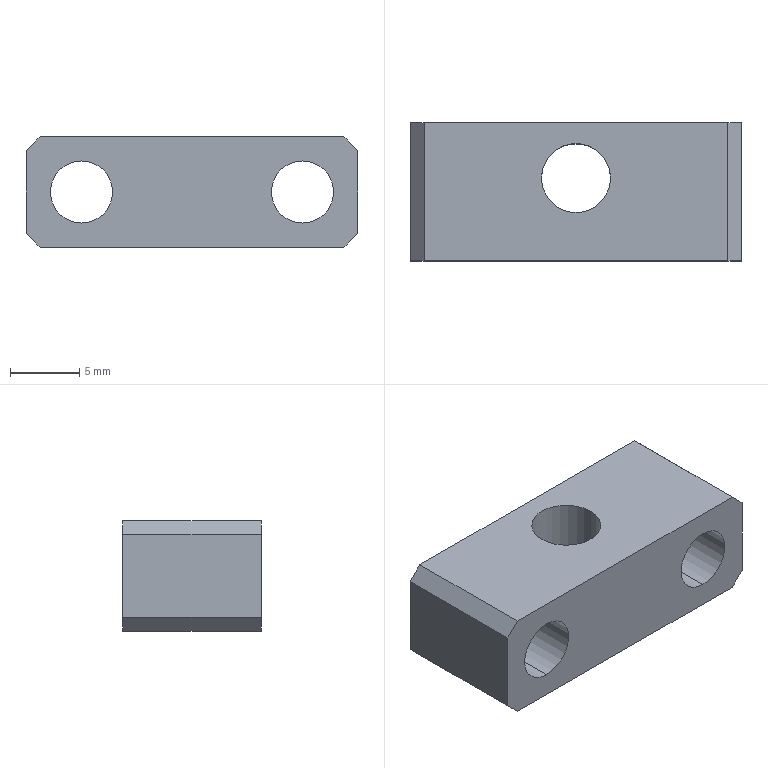Part | SolidWorks | features HoleWzd 2, Chamfer 1, Extrusion 1 | 1 solid | 16 faces | box 24 x 10 x 8 mm | volume 1425 mm3 | plane 10 | cylinder 6 | commonest cylinder face diameters 4.5 x4 5 x2
STEP:
#1=CARTESIAN_POINT('',(-2.5,1.,-4.));
#2=VERTEX_POINT('',#1);
#3=CARTESIAN_POINT('',(2.5,1.,-4.));
#4=VERTEX_POINT('',#3);
#5=CARTESIAN_POINT('',(0.,1.,-4.));
#6=DIRECTION('',(0.,0.,1.));
#7=DIRECTION('',(1.,0.,0.));
#8=AXIS2_PLACEMENT_3D('',#5,#6,#7);
#9=CIRCLE('',#8,2.5);
#10=EDGE_CURVE('',#2,#4,#9,.T.);
#11=ORIENTED_EDGE('',*,*,#10,.F.);
#12=CARTESIAN_POINT('',(-2.5,1.,4.));
#13=VERTEX_POINT('',#12);
#14=CARTESIAN_POINT('',(-2.5,1.,4.));
#15=DIRECTION('',(0.,0.,1.));
#16=VECTOR('',#15,1000.);
#17=LINE('',#14,#16);
#18=EDGE_CURVE('',#2,#13,#17,.T.);
#19=ORIENTED_EDGE('',*,*,#18,.T.);
#20=CARTESIAN_POINT('',(2.5,1.,4.));
#21=VERTEX_POINT('',#20);
#22=CARTESIAN_POINT('',(0.,1.,4.));
#23=DIRECTION('',(0.,0.,1.));
#24=DIRECTION('',(1.,0.,0.));
#25=AXIS2_PLACEMENT_3D('',#22,#23,#24);
#26=CIRCLE('',#25,2.5);
#27=EDGE_CURVE('',#13,#21,#26,.T.);
#28=ORIENTED_EDGE('',*,*,#27,.T.);
#29=CARTESIAN_POINT('',(2.5,1.,4.));
#30=DIRECTION('',(0.,0.,1.));
#31=VECTOR('',#30,1000.);
#32=LINE('',#29,#31);
#33=EDGE_CURVE('',#4,#21,#32,.T.);
#34=ORIENTED_EDGE('',*,*,#33,.F.);
#35=EDGE_LOOP('',(#11,#19,#28,#34));
#36=FACE_OUTER_BOUND('',#35,.T.);
#37=CARTESIAN_POINT('',(0.,1.,4.));
#38=DIRECTION('',(0.,0.,1.));
#39=DIRECTION('',(1.,0.,0.));
#40=AXIS2_PLACEMENT_3D('',#37,#38,#39);
#41=CYLINDRICAL_SURFACE('',#40,2.5);
#42=ADVANCED_FACE('',(#36),#41,.F.);
#43=CARTESIAN_POINT('',(-8.,-5.,-2.25));
#44=VERTEX_POINT('',#43);
#45=CARTESIAN_POINT('',(-8.,-5.,2.25));
#46=VERTEX_POINT('',#45);
#47=CARTESIAN_POINT('',(-8.,-5.,0.));
#48=DIRECTION('',(0.,1.,0.));
#49=DIRECTION('',(0.,0.,1.));
#50=AXIS2_PLACEMENT_3D('',#47,#48,#49);
#51=CIRCLE('',#50,2.25);
#52=EDGE_CURVE('',#44,#46,#51,.T.);
#53=ORIENTED_EDGE('',*,*,#52,.F.);
#54=CARTESIAN_POINT('',(-8.,5.,-2.25));
#55=VERTEX_POINT('',#54);
#56=CARTESIAN_POINT('',(-8.,5.,-2.25));
#57=DIRECTION('',(0.,1.,0.));
#58=VECTOR('',#57,1000.);
#59=LINE('',#56,#58);
#60=EDGE_CURVE('',#44,#55,#59,.T.);
#61=ORIENTED_EDGE('',*,*,#60,.T.);
#62=CARTESIAN_POINT('',(-8.,5.,2.25));
#63=VERTEX_POINT('',#62);
#64=CARTESIAN_POINT('',(-8.,5.,0.));
#65=DIRECTION('',(0.,1.,0.));
#66=DIRECTION('',(0.,0.,1.));
#67=AXIS2_PLACEMENT_3D('',#64,#65,#66);
#68=CIRCLE('',#67,2.25);
#69=EDGE_CURVE('',#55,#63,#68,.T.);
#70=ORIENTED_EDGE('',*,*,#69,.T.);
#71=CARTESIAN_POINT('',(-8.,5.,2.25));
#72=DIRECTION('',(0.,1.,0.));
#73=VECTOR('',#72,1000.);
#74=LINE('',#71,#73);
#75=EDGE_CURVE('',#46,#63,#74,.T.);
#76=ORIENTED_EDGE('',*,*,#75,.F.);
#77=EDGE_LOOP('',(#53,#61,#70,#76));
#78=FACE_OUTER_BOUND('',#77,.T.);
#79=CARTESIAN_POINT('',(-8.,5.,0.));
#80=DIRECTION('',(0.,1.,0.));
#81=DIRECTION('',(0.,0.,1.));
#82=AXIS2_PLACEMENT_3D('',#79,#80,#81);
#83=CYLINDRICAL_SURFACE('',#82,2.25);
#84=ADVANCED_FACE('',(#78),#83,.F.);
#85=CARTESIAN_POINT('',(8.,-5.,-2.25));
#86=VERTEX_POINT('',#85);
#87=CARTESIAN_POINT('',(8.,-5.,2.25));
#88=VERTEX_POINT('',#87);
#89=CARTESIAN_POINT('',(8.,-5.,0.));
#90=DIRECTION('',(0.,1.,0.));
#91=DIRECTION('',(0.,0.,1.));
#92=AXIS2_PLACEMENT_3D('',#89,#90,#91);
#93=CIRCLE('',#92,2.25);
#94=EDGE_CURVE('',#86,#88,#93,.T.);
#95=ORIENTED_EDGE('',*,*,#94,.F.);
#96=CARTESIAN_POINT('',(8.,5.,-2.25));
#97=VERTEX_POINT('',#96);
#98=CARTESIAN_POINT('',(8.,5.,-2.25));
#99=DIRECTION('',(0.,1.,0.));
#100=VECTOR('',#99,1000.);
#101=LINE('',#98,#100);
#102=EDGE_CURVE('',#86,#97,#101,.T.);
#103=ORIENTED_EDGE('',*,*,#102,.T.);
#104=CARTESIAN_POINT('',(8.,5.,2.25));
#105=VERTEX_POINT('',#104);
#106=CARTESIAN_POINT('',(8.,5.,0.));
#107=DIRECTION('',(0.,1.,0.));
#108=DIRECTION('',(0.,0.,1.));
#109=AXIS2_PLACEMENT_3D('',#106,#107,#108);
#110=CIRCLE('',#109,2.25);
#111=EDGE_CURVE('',#97,#105,#110,.T.);
#112=ORIENTED_EDGE('',*,*,#111,.T.);
#113=CARTESIAN_POINT('',(8.,5.,2.25));
#114=DIRECTION('',(0.,1.,0.));
#115=VECTOR('',#114,1000.);
#116=LINE('',#113,#115);
#117=EDGE_CURVE('',#88,#105,#116,.T.);
#118=ORIENTED_EDGE('',*,*,#117,.F.);
#119=EDGE_LOOP('',(#95,#103,#112,#118));
#120=FACE_OUTER_BOUND('',#119,.T.);
#121=CARTESIAN_POINT('',(8.,5.,0.));
#122=DIRECTION('',(0.,1.,0.));
#123=DIRECTION('',(0.,0.,1.));
#124=AXIS2_PLACEMENT_3D('',#121,#122,#123);
#125=CYLINDRICAL_SURFACE('',#124,2.25);
#126=ADVANCED_FACE('',(#120),#125,.F.);
#127=CARTESIAN_POINT('',(12.,-5.,3.));
#128=VERTEX_POINT('',#127);
#129=CARTESIAN_POINT('',(12.,-5.,-3.));
#130=VERTEX_POINT('',#129);
#131=CARTESIAN_POINT('',(12.,-5.,4.));
#132=DIRECTION('',(0.,0.,-1.));
#133=VECTOR('',#132,1000.);
#134=LINE('',#131,#133);
#135=EDGE_CURVE('',#128,#130,#134,.T.);
#136=ORIENTED_EDGE('',*,*,#135,.T.);
#137=CARTESIAN_POINT('',(12.,5.,-3.));
#138=VERTEX_POINT('',#137);
#139=CARTESIAN_POINT('',(12.,5.,-3.));
#140=DIRECTION('',(0.,1.,0.));
#141=VECTOR('',#140,1000.);
#142=LINE('',#139,#141);
#143=EDGE_CURVE('',#130,#138,#142,.T.);
#144=ORIENTED_EDGE('',*,*,#143,.T.);
#145=CARTESIAN_POINT('',(12.,5.,3.));
#146=VERTEX_POINT('',#145);
#147=CARTESIAN_POINT('',(12.,5.,4.));
#148=DIRECTION('',(0.,0.,-1.));
#149=VECTOR('',#148,1000.);
#150=LINE('',#147,#149);
#151=EDGE_CURVE('',#146,#138,#150,.T.);
#152=ORIENTED_EDGE('',*,*,#151,.F.);
#153=CARTESIAN_POINT('',(12.,-5.,3.));
#154=DIRECTION('',(0.,-1.,0.));
#155=VECTOR('',#154,1000.);
#156=LINE('',#153,#155);
#157=EDGE_CURVE('',#146,#128,#156,.T.);
#158=ORIENTED_EDGE('',*,*,#157,.T.);
#159=EDGE_LOOP('',(#136,#144,#152,#158));
#160=FACE_OUTER_BOUND('',#159,.T.);
#161=CARTESIAN_POINT('',(12.,5.,4.));
#162=DIRECTION('',(-1.,0.,0.));
#163=DIRECTION('',(0.,-1.,0.));
#164=AXIS2_PLACEMENT_3D('',#161,#162,#163);
#165=PLANE('',#164);
#166=ADVANCED_FACE('',(#160),#165,.F.);
#167=CARTESIAN_POINT('',(-8.,5.,0.));
#168=DIRECTION('',(0.,1.,0.));
#169=DIRECTION('',(0.,0.,1.));
#170=AXIS2_PLACEMENT_3D('',#167,#168,#169);
#171=CIRCLE('',#170,2.25);
#172=EDGE_CURVE('',#63,#55,#171,.T.);
#173=ORIENTED_EDGE('',*,*,#172,.F.);
#174=ORIENTED_EDGE('',*,*,#69,.F.);
#175=EDGE_LOOP('',(#173,#174));
#176=FACE_BOUND('',#175,.T.);
#177=CARTESIAN_POINT('',(8.,5.,0.));
#178=DIRECTION('',(0.,1.,0.));
#179=DIRECTION('',(0.,0.,1.));
#180=AXIS2_PLACEMENT_3D('',#177,#178,#179);
#181=CIRCLE('',#180,2.25);
#182=EDGE_CURVE('',#105,#97,#181,.T.);
#183=ORIENTED_EDGE('',*,*,#182,.F.);
#184=ORIENTED_EDGE('',*,*,#111,.F.);
#185=EDGE_LOOP('',(#183,#184));
#186=FACE_BOUND('',#185,.T.);
#187=CARTESIAN_POINT('',(11.,5.,-4.));
#188=VERTEX_POINT('',#187);
#189=CARTESIAN_POINT('',(-11.,5.,-4.));
#190=VERTEX_POINT('',#189);
#191=CARTESIAN_POINT('',(-12.,5.,-4.));
#192=DIRECTION('',(-1.,0.,0.));
#193=VECTOR('',#192,1000.);
#194=LINE('',#191,#193);
#195=EDGE_CURVE('',#188,#190,#194,.T.);
#196=ORIENTED_EDGE('',*,*,#195,.T.);
#197=CARTESIAN_POINT('',(-12.,5.,-3.));
#198=VERTEX_POINT('',#197);
#199=CARTESIAN_POINT('',(-12.,5.,-3.));
#200=DIRECTION('',(-0.7071,0.,0.7071));
#201=VECTOR('',#200,1000.);
#202=LINE('',#199,#201);
#203=EDGE_CURVE('',#190,#198,#202,.T.);
#204=ORIENTED_EDGE('',*,*,#203,.T.);
#205=CARTESIAN_POINT('',(-12.,5.,3.));
#206=VERTEX_POINT('',#205);
#207=CARTESIAN_POINT('',(-12.,5.,4.));
#208=DIRECTION('',(0.,0.,-1.));
#209=VECTOR('',#208,1000.);
#210=LINE('',#207,#209);
#211=EDGE_CURVE('',#206,#198,#210,.T.);
#212=ORIENTED_EDGE('',*,*,#211,.F.);
#213=CARTESIAN_POINT('',(-11.,5.,4.));
#214=VERTEX_POINT('',#213);
#215=CARTESIAN_POINT('',(-11.,5.,4.));
#216=DIRECTION('',(0.7071,0.,0.7071));
#217=VECTOR('',#216,1000.);
#218=LINE('',#215,#217);
#219=EDGE_CURVE('',#206,#214,#218,.T.);
#220=ORIENTED_EDGE('',*,*,#219,.T.);
#221=CARTESIAN_POINT('',(11.,5.,4.));
#222=VERTEX_POINT('',#221);
#223=CARTESIAN_POINT('',(-12.,5.,4.));
#224=DIRECTION('',(-1.,0.,0.));
#225=VECTOR('',#224,1000.);
#226=LINE('',#223,#225);
#227=EDGE_CURVE('',#222,#214,#226,.T.);
#228=ORIENTED_EDGE('',*,*,#227,.F.);
#229=CARTESIAN_POINT('',(11.,5.,4.));
#230=DIRECTION('',(0.7071,0.,-0.7071));
#231=VECTOR('',#230,1000.);
#232=LINE('',#229,#231);
#233=EDGE_CURVE('',#222,#146,#232,.T.);
#234=ORIENTED_EDGE('',*,*,#233,.T.);
#235=ORIENTED_EDGE('',*,*,#151,.T.);
#236=CARTESIAN_POINT('',(12.,5.,-3.));
#237=DIRECTION('',(-0.7071,0.,-0.7071));
#238=VECTOR('',#237,1000.);
#239=LINE('',#236,#238);
#240=EDGE_CURVE('',#138,#188,#239,.T.);
#241=ORIENTED_EDGE('',*,*,#240,.T.);
#242=EDGE_LOOP('',(#196,#204,#212,#220,#228,#234,#235,#241));
#243=FACE_OUTER_BOUND('',#242,.T.);
#244=CARTESIAN_POINT('',(-12.,5.,4.));
#245=DIRECTION('',(0.,-1.,0.));
#246=DIRECTION('',(0.,0.,-1.));
#247=AXIS2_PLACEMENT_3D('',#244,#245,#246);
#248=PLANE('',#247);
#249=ADVANCED_FACE('',(#176,#186,#243),#248,.F.);
#250=ORIENTED_EDGE('',*,*,#211,.T.);
#251=CARTESIAN_POINT('',(-12.,-5.,-3.));
#252=VERTEX_POINT('',#251);
#253=CARTESIAN_POINT('',(-12.,5.,-3.));
#254=DIRECTION('',(0.,-1.,0.));
#255=VECTOR('',#254,1000.);
#256=LINE('',#253,#255);
#257=EDGE_CURVE('',#198,#252,#256,.T.);
#258=ORIENTED_EDGE('',*,*,#257,.T.);
#259=CARTESIAN_POINT('',(-12.,-5.,3.));
#260=VERTEX_POINT('',#259);
#261=CARTESIAN_POINT('',(-12.,-5.,4.));
#262=DIRECTION('',(0.,0.,-1.));
#263=VECTOR('',#262,1000.);
#264=LINE('',#261,#263);
#265=EDGE_CURVE('',#260,#252,#264,.T.);
#266=ORIENTED_EDGE('',*,*,#265,.F.);
#267=CARTESIAN_POINT('',(-12.,5.,3.));
#268=DIRECTION('',(0.,1.,0.));
#269=VECTOR('',#268,1000.);
#270=LINE('',#267,#269);
#271=EDGE_CURVE('',#260,#206,#270,.T.);
#272=ORIENTED_EDGE('',*,*,#271,.T.);
#273=EDGE_LOOP('',(#250,#258,#266,#272));
#274=FACE_OUTER_BOUND('',#273,.T.);
#275=CARTESIAN_POINT('',(-12.,5.,4.));
#276=DIRECTION('',(1.,0.,0.));
#277=DIRECTION('',(0.,1.,0.));
#278=AXIS2_PLACEMENT_3D('',#275,#276,#277);
#279=PLANE('',#278);
#280=ADVANCED_FACE('',(#274),#279,.F.);
#281=CARTESIAN_POINT('',(-8.,-5.,0.));
#282=DIRECTION('',(0.,1.,0.));
#283=DIRECTION('',(0.,0.,1.));
#284=AXIS2_PLACEMENT_3D('',#281,#282,#283);
#285=CIRCLE('',#284,2.25);
#286=EDGE_CURVE('',#46,#44,#285,.T.);
#287=ORIENTED_EDGE('',*,*,#286,.T.);
#288=ORIENTED_EDGE('',*,*,#52,.T.);
#289=EDGE_LOOP('',(#287,#288));
#290=FACE_BOUND('',#289,.T.);
#291=CARTESIAN_POINT('',(8.,-5.,0.));
#292=DIRECTION('',(0.,1.,0.));
#293=DIRECTION('',(0.,0.,1.));
#294=AXIS2_PLACEMENT_3D('',#291,#292,#293);
#295=CIRCLE('',#294,2.25);
#296=EDGE_CURVE('',#88,#86,#295,.T.);
#297=ORIENTED_EDGE('',*,*,#296,.T.);
#298=ORIENTED_EDGE('',*,*,#94,.T.);
#299=EDGE_LOOP('',(#297,#298));
#300=FACE_BOUND('',#299,.T.);
#301=ORIENTED_EDGE('',*,*,#265,.T.);
#302=CARTESIAN_POINT('',(-11.,-5.,-4.));
#303=VERTEX_POINT('',#302);
#304=CARTESIAN_POINT('',(-12.,-5.,-3.));
#305=DIRECTION('',(0.7071,0.,-0.7071));
#306=VECTOR('',#305,1000.);
#307=LINE('',#304,#306);
#308=EDGE_CURVE('',#252,#303,#307,.T.);
#309=ORIENTED_EDGE('',*,*,#308,.T.);
#310=CARTESIAN_POINT('',(11.,-5.,-4.));
#311=VERTEX_POINT('',#310);
#312=CARTESIAN_POINT('',(-12.,-5.,-4.));
#313=DIRECTION('',(1.,0.,0.));
#314=VECTOR('',#313,1000.);
#315=LINE('',#312,#314);
#316=EDGE_CURVE('',#303,#311,#315,.T.);
#317=ORIENTED_EDGE('',*,*,#316,.T.);
#318=CARTESIAN_POINT('',(12.,-5.,-3.));
#319=DIRECTION('',(0.7071,0.,0.7071));
#320=VECTOR('',#319,1000.);
#321=LINE('',#318,#320);
#322=EDGE_CURVE('',#311,#130,#321,.T.);
#323=ORIENTED_EDGE('',*,*,#322,.T.);
#324=ORIENTED_EDGE('',*,*,#135,.F.);
#325=CARTESIAN_POINT('',(11.,-5.,4.));
#326=VERTEX_POINT('',#325);
#327=CARTESIAN_POINT('',(11.,-5.,4.));
#328=DIRECTION('',(-0.7071,0.,0.7071));
#329=VECTOR('',#328,1000.);
#330=LINE('',#327,#329);
#331=EDGE_CURVE('',#128,#326,#330,.T.);
#332=ORIENTED_EDGE('',*,*,#331,.T.);
#333=CARTESIAN_POINT('',(-11.,-5.,4.));
#334=VERTEX_POINT('',#333);
#335=CARTESIAN_POINT('',(-12.,-5.,4.));
#336=DIRECTION('',(1.,0.,0.));
#337=VECTOR('',#336,1000.);
#338=LINE('',#335,#337);
#339=EDGE_CURVE('',#334,#326,#338,.T.);
#340=ORIENTED_EDGE('',*,*,#339,.F.);
#341=CARTESIAN_POINT('',(-11.,-5.,4.));
#342=DIRECTION('',(-0.7071,0.,-0.7071));
#343=VECTOR('',#342,1000.);
#344=LINE('',#341,#343);
#345=EDGE_CURVE('',#334,#260,#344,.T.);
#346=ORIENTED_EDGE('',*,*,#345,.T.);
#347=EDGE_LOOP('',(#301,#309,#317,#323,#324,#332,#340,#346));
#348=FACE_OUTER_BOUND('',#347,.T.);
#349=CARTESIAN_POINT('',(-12.,-5.,4.));
#350=DIRECTION('',(0.,1.,0.));
#351=DIRECTION('',(0.,0.,1.));
#352=AXIS2_PLACEMENT_3D('',#349,#350,#351);
#353=PLANE('',#352);
#354=ADVANCED_FACE('',(#290,#300,#348),#353,.F.);
#355=CARTESIAN_POINT('',(0.,1.,4.));
#356=DIRECTION('',(0.,0.,1.));
#357=DIRECTION('',(1.,0.,0.));
#358=AXIS2_PLACEMENT_3D('',#355,#356,#357);
#359=CIRCLE('',#358,2.5);
#360=EDGE_CURVE('',#21,#13,#359,.T.);
#361=ORIENTED_EDGE('',*,*,#360,.F.);
#362=ORIENTED_EDGE('',*,*,#27,.F.);
#363=EDGE_LOOP('',(#361,#362));
#364=FACE_BOUND('',#363,.T.);
#365=ORIENTED_EDGE('',*,*,#339,.T.);
#366=CARTESIAN_POINT('',(11.,5.,4.));
#367=DIRECTION('',(0.,1.,0.));
#368=VECTOR('',#367,1000.);
#369=LINE('',#366,#368);
#370=EDGE_CURVE('',#326,#222,#369,.T.);
#371=ORIENTED_EDGE('',*,*,#370,.T.);
#372=ORIENTED_EDGE('',*,*,#227,.T.);
#373=CARTESIAN_POINT('',(-11.,-5.,4.));
#374=DIRECTION('',(0.,-1.,0.));
#375=VECTOR('',#374,1000.);
#376=LINE('',#373,#375);
#377=EDGE_CURVE('',#214,#334,#376,.T.);
#378=ORIENTED_EDGE('',*,*,#377,.T.);
#379=EDGE_LOOP('',(#365,#371,#372,#378));
#380=FACE_OUTER_BOUND('',#379,.T.);
#381=CARTESIAN_POINT('',(0.,0.,4.));
#382=DIRECTION('',(0.,0.,1.));
#383=DIRECTION('',(1.,0.,0.));
#384=AXIS2_PLACEMENT_3D('',#381,#382,#383);
#385=PLANE('',#384);
#386=ADVANCED_FACE('',(#364,#380),#385,.T.);
#387=CARTESIAN_POINT('',(0.,1.,-4.));
#388=DIRECTION('',(0.,0.,1.));
#389=DIRECTION('',(1.,0.,0.));
#390=AXIS2_PLACEMENT_3D('',#387,#388,#389);
#391=CIRCLE('',#390,2.5);
#392=EDGE_CURVE('',#4,#2,#391,.T.);
#393=ORIENTED_EDGE('',*,*,#392,.T.);
#394=ORIENTED_EDGE('',*,*,#10,.T.);
#395=EDGE_LOOP('',(#393,#394));
#396=FACE_BOUND('',#395,.T.);
#397=ORIENTED_EDGE('',*,*,#316,.F.);
#398=CARTESIAN_POINT('',(-11.,0.,-4.));
#399=DIRECTION('',(0.,1.,0.));
#400=VECTOR('',#399,1000.);
#401=LINE('',#398,#400);
#402=EDGE_CURVE('',#303,#190,#401,.T.);
#403=ORIENTED_EDGE('',*,*,#402,.T.);
#404=ORIENTED_EDGE('',*,*,#195,.F.);
#405=CARTESIAN_POINT('',(11.,0.,-4.));
#406=DIRECTION('',(0.,-1.,0.));
#407=VECTOR('',#406,1000.);
#408=LINE('',#405,#407);
#409=EDGE_CURVE('',#188,#311,#408,.T.);
#410=ORIENTED_EDGE('',*,*,#409,.T.);
#411=EDGE_LOOP('',(#397,#403,#404,#410));
#412=FACE_OUTER_BOUND('',#411,.T.);
#413=CARTESIAN_POINT('',(0.,0.,-4.));
#414=DIRECTION('',(0.,0.,1.));
#415=DIRECTION('',(1.,0.,0.));
#416=AXIS2_PLACEMENT_3D('',#413,#414,#415);
#417=PLANE('',#416);
#418=ADVANCED_FACE('',(#396,#412),#417,.F.);
#419=ORIENTED_EDGE('',*,*,#102,.F.);
#420=ORIENTED_EDGE('',*,*,#296,.F.);
#421=ORIENTED_EDGE('',*,*,#117,.T.);
#422=ORIENTED_EDGE('',*,*,#182,.T.);
#423=EDGE_LOOP('',(#419,#420,#421,#422));
#424=FACE_OUTER_BOUND('',#423,.T.);
#425=CARTESIAN_POINT('',(8.,5.,0.));
#426=DIRECTION('',(0.,1.,0.));
#427=DIRECTION('',(0.,0.,1.));
#428=AXIS2_PLACEMENT_3D('',#425,#426,#427);
#429=CYLINDRICAL_SURFACE('',#428,2.25);
#430=ADVANCED_FACE('',(#424),#429,.F.);
#431=ORIENTED_EDGE('',*,*,#60,.F.);
#432=ORIENTED_EDGE('',*,*,#286,.F.);
#433=ORIENTED_EDGE('',*,*,#75,.T.);
#434=ORIENTED_EDGE('',*,*,#172,.T.);
#435=EDGE_LOOP('',(#431,#432,#433,#434));
#436=FACE_OUTER_BOUND('',#435,.T.);
#437=CARTESIAN_POINT('',(-8.,5.,0.));
#438=DIRECTION('',(0.,1.,0.));
#439=DIRECTION('',(0.,0.,1.));
#440=AXIS2_PLACEMENT_3D('',#437,#438,#439);
#441=CYLINDRICAL_SURFACE('',#440,2.25);
#442=ADVANCED_FACE('',(#436),#441,.F.);
#443=ORIENTED_EDGE('',*,*,#203,.F.);
#444=ORIENTED_EDGE('',*,*,#402,.F.);
#445=ORIENTED_EDGE('',*,*,#308,.F.);
#446=ORIENTED_EDGE('',*,*,#257,.F.);
#447=EDGE_LOOP('',(#443,#444,#445,#446));
#448=FACE_OUTER_BOUND('',#447,.T.);
#449=CARTESIAN_POINT('',(-12.,5.,-3.));
#450=DIRECTION('',(0.7071,0.,0.7071));
#451=DIRECTION('',(0.,-1.,0.));
#452=AXIS2_PLACEMENT_3D('',#449,#450,#451);
#453=PLANE('',#452);
#454=ADVANCED_FACE('',(#448),#453,.F.);
#455=ORIENTED_EDGE('',*,*,#322,.F.);
#456=ORIENTED_EDGE('',*,*,#409,.F.);
#457=ORIENTED_EDGE('',*,*,#240,.F.);
#458=ORIENTED_EDGE('',*,*,#143,.F.);
#459=EDGE_LOOP('',(#455,#456,#457,#458));
#460=FACE_OUTER_BOUND('',#459,.T.);
#461=CARTESIAN_POINT('',(12.,5.,-3.));
#462=DIRECTION('',(-0.7071,0.,0.7071));
#463=DIRECTION('',(0.,1.,0.));
#464=AXIS2_PLACEMENT_3D('',#461,#462,#463);
#465=PLANE('',#464);
#466=ADVANCED_FACE('',(#460),#465,.F.);
#467=ORIENTED_EDGE('',*,*,#331,.F.);
#468=ORIENTED_EDGE('',*,*,#157,.F.);
#469=ORIENTED_EDGE('',*,*,#233,.F.);
#470=ORIENTED_EDGE('',*,*,#370,.F.);
#471=EDGE_LOOP('',(#467,#468,#469,#470));
#472=FACE_OUTER_BOUND('',#471,.T.);
#473=CARTESIAN_POINT('',(11.,0.,4.));
#474=DIRECTION('',(0.7071,0.,0.7071));
#475=DIRECTION('',(0.,-1.,0.));
#476=AXIS2_PLACEMENT_3D('',#473,#474,#475);
#477=PLANE('',#476);
#478=ADVANCED_FACE('',(#472),#477,.T.);
#479=ORIENTED_EDGE('',*,*,#219,.F.);
#480=ORIENTED_EDGE('',*,*,#271,.F.);
#481=ORIENTED_EDGE('',*,*,#345,.F.);
#482=ORIENTED_EDGE('',*,*,#377,.F.);
#483=EDGE_LOOP('',(#479,#480,#481,#482));
#484=FACE_OUTER_BOUND('',#483,.T.);
#485=CARTESIAN_POINT('',(-11.,0.,4.));
#486=DIRECTION('',(-0.7071,0.,0.7071));
#487=DIRECTION('',(0.,1.,0.));
#488=AXIS2_PLACEMENT_3D('',#485,#486,#487);
#489=PLANE('',#488);
#490=ADVANCED_FACE('',(#484),#489,.T.);
#491=ORIENTED_EDGE('',*,*,#18,.F.);
#492=ORIENTED_EDGE('',*,*,#392,.F.);
#493=ORIENTED_EDGE('',*,*,#33,.T.);
#494=ORIENTED_EDGE('',*,*,#360,.T.);
#495=EDGE_LOOP('',(#491,#492,#493,#494));
#496=FACE_OUTER_BOUND('',#495,.T.);
#497=CARTESIAN_POINT('',(0.,1.,4.));
#498=DIRECTION('',(0.,0.,1.));
#499=DIRECTION('',(1.,0.,0.));
#500=AXIS2_PLACEMENT_3D('',#497,#498,#499);
#501=CYLINDRICAL_SURFACE('',#500,2.5);
#502=ADVANCED_FACE('',(#496),#501,.F.);
#503=CLOSED_SHELL('',(#42,#84,#126,#166,#249,#280,#354,#386,#418,#430,#442,#454,#466,#478,#490,#502));
#504=MANIFOLD_SOLID_BREP('',#503);
#505=CARTESIAN_POINT('',(0.,0.,0.));
#506=DIRECTION('',(0.,0.,1.));
#507=DIRECTION('',(1.,0.,0.));
#508=AXIS2_PLACEMENT_3D('',#505,#506,#507);
#509=(LENGTH_UNIT()NAMED_UNIT(*)SI_UNIT(.MILLI.,.METRE.));
#510=UNCERTAINTY_MEASURE_WITH_UNIT(LENGTH_MEASURE(0.00001),#509,'','');
#511=(NAMED_UNIT(*)PLANE_ANGLE_UNIT()SI_UNIT($,.RADIAN.));
#512=(NAMED_UNIT(*)SI_UNIT($,.STERADIAN.)SOLID_ANGLE_UNIT());
#513=(GEOMETRIC_REPRESENTATION_CONTEXT(3)GLOBAL_UNCERTAINTY_ASSIGNED_CONTEXT((#510))GLOBAL_UNIT_ASSIGNED_CONTEXT((#509,#511,#512))REPRESENTATION_CONTEXT('',''));
#514=ADVANCED_BREP_SHAPE_REPRESENTATION('',(#504,#508),#513);